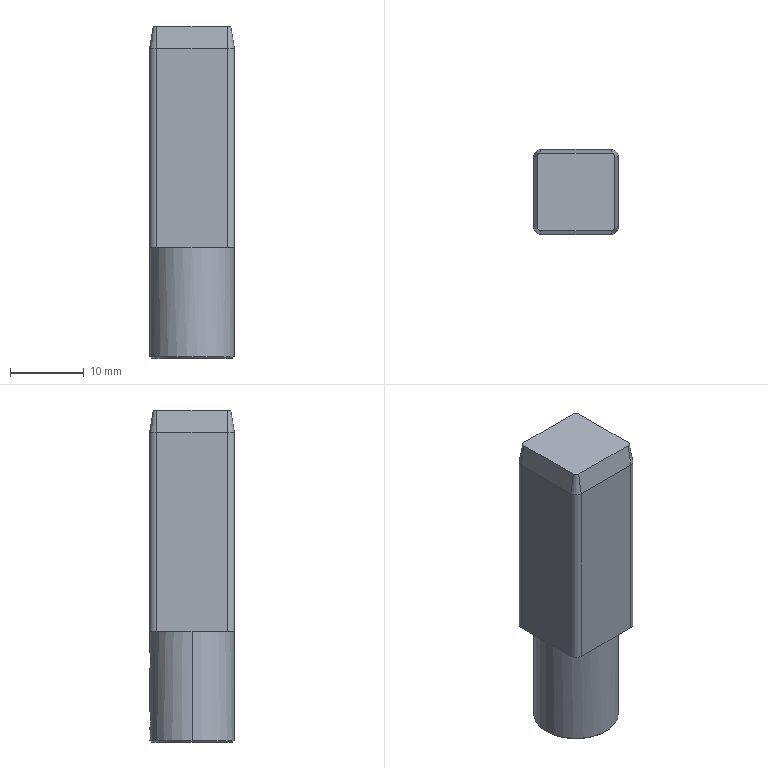Part | STEP file | PN_0001 Rotating Shaft Adapter Block | 1 solid | 35 faces | box 11.5 x 11.5 x 45 mm | volume 4695 mm3 | plane 15 | cylinder 12 | cone 8 | commonest cylinder face diameters 2 x4 2.5 x4 8 x2 11.5 x2